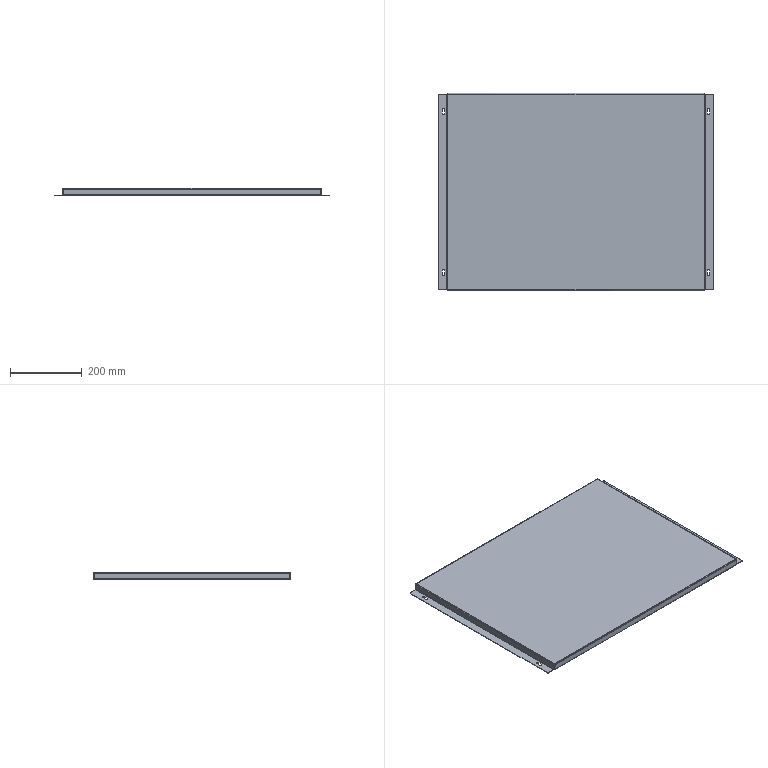Part | NX | 1 solid | 90 faces | box 767 x 550 x 20 mm | volume 736610 mm3 | plane 54 | cylinder 28 | spline 8 | commonest cylinder face diameters 1.5 x8 4.5 x8 7 x8 6 x4